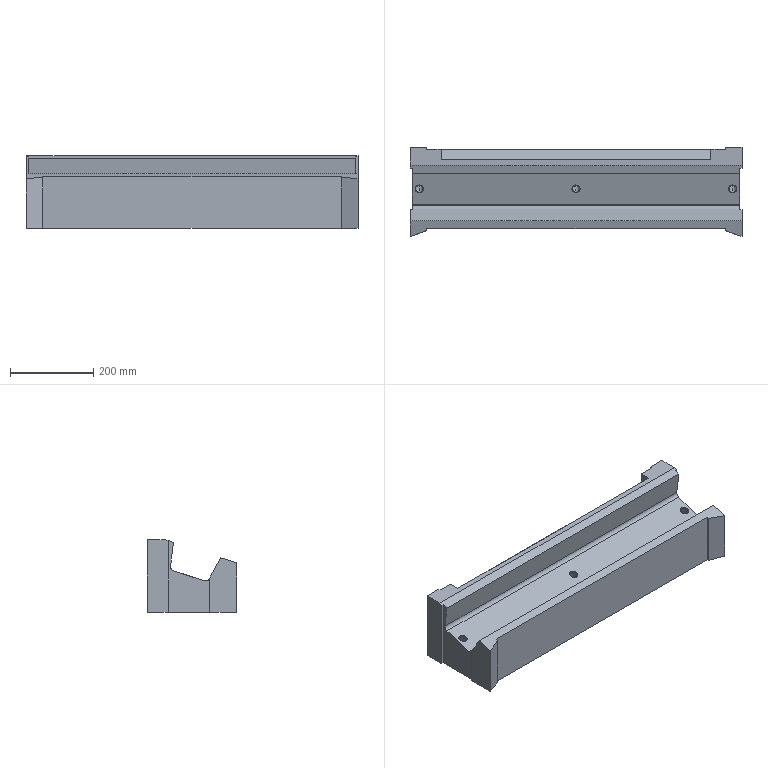Part | SolidWorks | features ICE 5, 3DProfileFeature 2, HoleWzd 2, Extrusion 1, Fillet 1, MirrorPattern 1 | 1 solid | 77 faces | box 800 x 215 x 175 mm | volume 15797212 mm3 | plane 50 | cone 16 | cylinder 11 | commonest cylinder face diameters 17.5 x8 20 x3